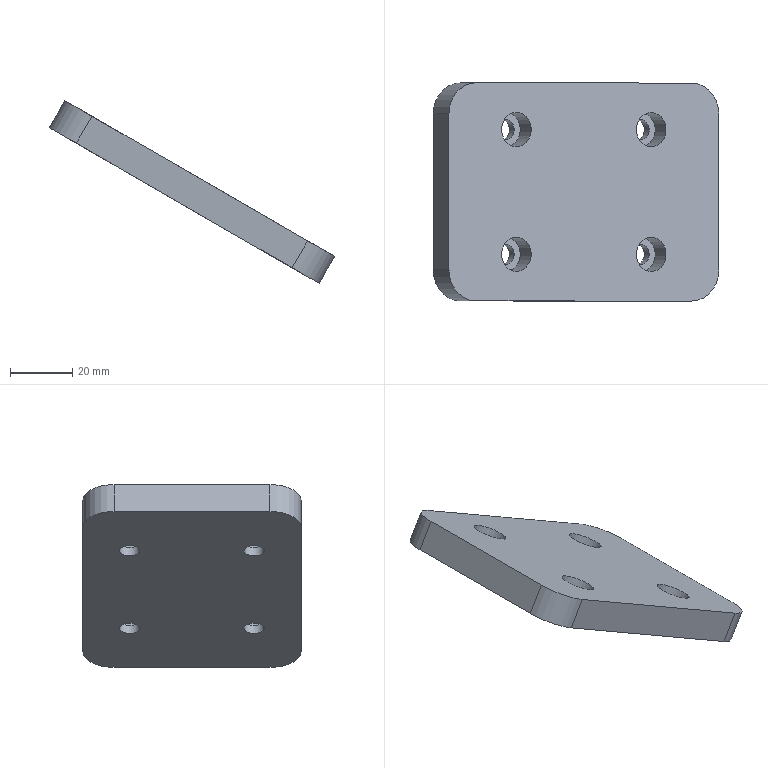Part | STEP file | solid 242 | 1 solid | 22 faces | box 91.603 x 70 x 58.66 mm | volume 66082 mm3 | cylinder 12 | plane 10 | commonest cylinder face diameters 6.5 x4 11 x4 20 x4